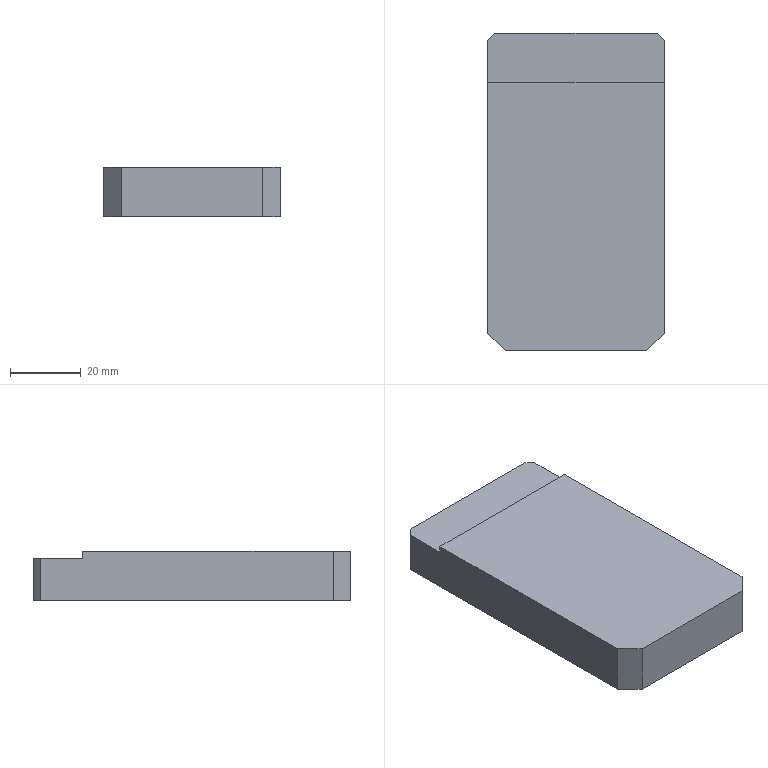Part | STEP file | Backup 2012-3-22-014 | 1 solid | 12 faces | box 50 x 90 x 14 mm | volume 61202 mm3 | plane 12
STEP:
#1=CARTESIAN_POINT('',(0.,0.,0.));
#2=DIRECTION('',(0.,0.,1.));
#3=DIRECTION('',(1.,0.,0.));
#4=AXIS2_PLACEMENT_3D('',#1,#2,#3);
#5=CARTESIAN_POINT('',(23.,45.,12.));
#6=VERTEX_POINT('',#5);
#7=CARTESIAN_POINT('',(-23.,45.,12.));
#8=VERTEX_POINT('',#7);
#9=CARTESIAN_POINT('',(-25.,45.,12.));
#10=DIRECTION('',(-1.,0.,0.));
#11=VECTOR('',#10,1.);
#12=LINE('',#9,#11);
#13=CARTESIAN_POINT('',(-25.,45.,14.));
#14=DIRECTION('',(0.,-1.,0.));
#15=DIRECTION('',(0.,0.,-1.));
#16=AXIS2_PLACEMENT_3D('',#13,#14,#15);
#17=PLANE('',#16);
#18=CARTESIAN_POINT('',(2.,0.));
#19=DIRECTION('',(0.,-1.));
#20=VECTOR('',#19,1.);
#21=LINE('',#18,#20);
#22=(GEOMETRIC_REPRESENTATION_CONTEXT(2)PARAMETRIC_REPRESENTATION_CONTEXT()REPRESENTATION_CONTEXT('',''));
#23=DEFINITIONAL_REPRESENTATION('',(#21),#22);
#24=PCURVE('',#17,#23);
#25=CARTESIAN_POINT('',(-25.,31.,12.));
#26=DIRECTION('',(0.,0.,1.));
#27=DIRECTION('',(1.,0.,0.));
#28=AXIS2_PLACEMENT_3D('',#25,#26,#27);
#29=PLANE('',#28);
#30=CARTESIAN_POINT('',(0.,14.));
#31=DIRECTION('',(-1.,0.));
#32=VECTOR('',#31,1.);
#33=LINE('',#30,#32);
#34=(GEOMETRIC_REPRESENTATION_CONTEXT(2)PARAMETRIC_REPRESENTATION_CONTEXT()REPRESENTATION_CONTEXT('',''));
#35=DEFINITIONAL_REPRESENTATION('',(#33),#34);
#36=PCURVE('',#29,#35);
#37=SURFACE_CURVE('',#12,(#24,#36),.PCURVE_S1.);
#38=EDGE_CURVE('',#6,#8,#37,.T.);
#39=ORIENTED_EDGE('',*,*,#38,.F.);
#40=CARTESIAN_POINT('',(23.,45.,0.));
#41=VERTEX_POINT('',#40);
#42=CARTESIAN_POINT('',(23.,45.,14.));
#43=DIRECTION('',(0.,0.,-1.));
#44=VECTOR('',#43,1.);
#45=LINE('',#42,#44);
#46=CARTESIAN_POINT('',(0.,48.));
#47=DIRECTION('',(1.,0.));
#48=VECTOR('',#47,1.);
#49=LINE('',#46,#48);
#50=(GEOMETRIC_REPRESENTATION_CONTEXT(2)PARAMETRIC_REPRESENTATION_CONTEXT()REPRESENTATION_CONTEXT('',''));
#51=DEFINITIONAL_REPRESENTATION('',(#49),#50);
#52=PCURVE('',#17,#51);
#53=CARTESIAN_POINT('',(23.,45.,14.));
#54=DIRECTION('',(-0.7071,-0.7071,0.));
#55=DIRECTION('',(0.7071,-0.7071,0.));
#56=AXIS2_PLACEMENT_3D('',#53,#54,#55);
#57=PLANE('',#56);
#58=CARTESIAN_POINT('',(0.,0.));
#59=DIRECTION('',(0.,-1.));
#60=VECTOR('',#59,1.);
#61=LINE('',#58,#60);
#62=(GEOMETRIC_REPRESENTATION_CONTEXT(2)PARAMETRIC_REPRESENTATION_CONTEXT()REPRESENTATION_CONTEXT('',''));
#63=DEFINITIONAL_REPRESENTATION('',(#61),#62);
#64=PCURVE('',#57,#63);
#65=SURFACE_CURVE('',#45,(#52,#64),.PCURVE_S1.);
#66=EDGE_CURVE('',#6,#41,#65,.T.);
#67=ORIENTED_EDGE('',*,*,#66,.T.);
#68=CARTESIAN_POINT('',(-23.,45.,0.));
#69=VERTEX_POINT('',#68);
#70=CARTESIAN_POINT('',(-25.,45.,0.));
#71=DIRECTION('',(-1.,0.,0.));
#72=VECTOR('',#71,1.);
#73=LINE('',#70,#72);
#74=CARTESIAN_POINT('',(14.,0.));
#75=DIRECTION('',(0.,-1.));
#76=VECTOR('',#75,1.);
#77=LINE('',#74,#76);
#78=(GEOMETRIC_REPRESENTATION_CONTEXT(2)PARAMETRIC_REPRESENTATION_CONTEXT()REPRESENTATION_CONTEXT('',''));
#79=DEFINITIONAL_REPRESENTATION('',(#77),#78);
#80=PCURVE('',#17,#79);
#81=CARTESIAN_POINT('',(25.,-45.,0.));
#82=DIRECTION('',(0.,0.,1.));
#83=DIRECTION('',(1.,0.,0.));
#84=AXIS2_PLACEMENT_3D('',#81,#82,#83);
#85=PLANE('',#84);
#86=CARTESIAN_POINT('',(-50.,90.));
#87=DIRECTION('',(-1.,0.));
#88=VECTOR('',#87,1.);
#89=LINE('',#86,#88);
#90=(GEOMETRIC_REPRESENTATION_CONTEXT(2)PARAMETRIC_REPRESENTATION_CONTEXT()REPRESENTATION_CONTEXT('',''));
#91=DEFINITIONAL_REPRESENTATION('',(#89),#90);
#92=PCURVE('',#85,#91);
#93=SURFACE_CURVE('',#73,(#80,#92),.PCURVE_S1.);
#94=EDGE_CURVE('',#41,#69,#93,.T.);
#95=ORIENTED_EDGE('',*,*,#94,.T.);
#96=CARTESIAN_POINT('',(-23.,45.,14.));
#97=DIRECTION('',(0.,0.,1.));
#98=VECTOR('',#97,1.);
#99=LINE('',#96,#98);
#100=CARTESIAN_POINT('',(0.,2.));
#101=DIRECTION('',(-1.,0.));
#102=VECTOR('',#101,1.);
#103=LINE('',#100,#102);
#104=(GEOMETRIC_REPRESENTATION_CONTEXT(2)PARAMETRIC_REPRESENTATION_CONTEXT()REPRESENTATION_CONTEXT('',''));
#105=DEFINITIONAL_REPRESENTATION('',(#103),#104);
#106=PCURVE('',#17,#105);
#107=CARTESIAN_POINT('',(-25.,43.,14.));
#108=DIRECTION('',(0.7071,-0.7071,0.));
#109=DIRECTION('',(0.7071,0.7071,0.));
#110=AXIS2_PLACEMENT_3D('',#107,#108,#109);
#111=PLANE('',#110);
#112=CARTESIAN_POINT('',(2.828,0.));
#113=DIRECTION('',(0.,1.));
#114=VECTOR('',#113,1.);
#115=LINE('',#112,#114);
#116=(GEOMETRIC_REPRESENTATION_CONTEXT(2)PARAMETRIC_REPRESENTATION_CONTEXT()REPRESENTATION_CONTEXT('',''));
#117=DEFINITIONAL_REPRESENTATION('',(#115),#116);
#118=PCURVE('',#111,#117);
#119=SURFACE_CURVE('',#99,(#106,#118),.PCURVE_S1.);
#120=EDGE_CURVE('',#69,#8,#119,.T.);
#121=ORIENTED_EDGE('',*,*,#120,.T.);
#122=EDGE_LOOP('',(#39,#67,#95,#121));
#123=FACE_BOUND('',#122,.T.);
#124=ADVANCED_FACE('',(#123),#17,.F.);
#125=CARTESIAN_POINT('',(25.,-40.,0.));
#126=VERTEX_POINT('',#125);
#127=CARTESIAN_POINT('',(25.,43.,0.));
#128=VERTEX_POINT('',#127);
#129=CARTESIAN_POINT('',(25.,45.,0.));
#130=DIRECTION('',(0.,1.,0.));
#131=VECTOR('',#130,1.);
#132=LINE('',#129,#131);
#133=CARTESIAN_POINT('',(25.,45.,14.));
#134=DIRECTION('',(-1.,0.,0.));
#135=DIRECTION('',(0.,-1.,0.));
#136=AXIS2_PLACEMENT_3D('',#133,#134,#135);
#137=PLANE('',#136);
#138=CARTESIAN_POINT('',(0.,-14.));
#139=DIRECTION('',(-1.,0.));
#140=VECTOR('',#139,1.);
#141=LINE('',#138,#140);
#142=(GEOMETRIC_REPRESENTATION_CONTEXT(2)PARAMETRIC_REPRESENTATION_CONTEXT()REPRESENTATION_CONTEXT('',''));
#143=DEFINITIONAL_REPRESENTATION('',(#141),#142);
#144=PCURVE('',#137,#143);
#145=CARTESIAN_POINT('',(0.,90.));
#146=DIRECTION('',(0.,1.));
#147=VECTOR('',#146,1.);
#148=LINE('',#145,#147);
#149=(GEOMETRIC_REPRESENTATION_CONTEXT(2)PARAMETRIC_REPRESENTATION_CONTEXT()REPRESENTATION_CONTEXT('',''));
#150=DEFINITIONAL_REPRESENTATION('',(#148),#149);
#151=PCURVE('',#85,#150);
#152=SURFACE_CURVE('',#132,(#144,#151),.PCURVE_S1.);
#153=EDGE_CURVE('',#126,#128,#152,.T.);
#154=ORIENTED_EDGE('',*,*,#153,.T.);
#155=CARTESIAN_POINT('',(25.,43.,12.));
#156=VERTEX_POINT('',#155);
#157=CARTESIAN_POINT('',(25.,43.,14.));
#158=DIRECTION('',(0.,0.,1.));
#159=VECTOR('',#158,1.);
#160=LINE('',#157,#159);
#161=CARTESIAN_POINT('',(2.,0.));
#162=DIRECTION('',(0.,1.));
#163=VECTOR('',#162,1.);
#164=LINE('',#161,#163);
#165=(GEOMETRIC_REPRESENTATION_CONTEXT(2)PARAMETRIC_REPRESENTATION_CONTEXT()REPRESENTATION_CONTEXT('',''));
#166=DEFINITIONAL_REPRESENTATION('',(#164),#165);
#167=PCURVE('',#137,#166);
#168=CARTESIAN_POINT('',(2.828,0.));
#169=DIRECTION('',(0.,1.));
#170=VECTOR('',#169,1.);
#171=LINE('',#168,#170);
#172=(GEOMETRIC_REPRESENTATION_CONTEXT(2)PARAMETRIC_REPRESENTATION_CONTEXT()REPRESENTATION_CONTEXT('',''));
#173=DEFINITIONAL_REPRESENTATION('',(#171),#172);
#174=PCURVE('',#57,#173);
#175=SURFACE_CURVE('',#160,(#167,#174),.PCURVE_S1.);
#176=EDGE_CURVE('',#128,#156,#175,.T.);
#177=ORIENTED_EDGE('',*,*,#176,.T.);
#178=CARTESIAN_POINT('',(25.,31.,12.));
#179=VERTEX_POINT('',#178);
#180=CARTESIAN_POINT('',(25.,45.,12.));
#181=DIRECTION('',(0.,1.,0.));
#182=VECTOR('',#181,1.);
#183=LINE('',#180,#182);
#184=CARTESIAN_POINT('',(0.,-2.));
#185=DIRECTION('',(-1.,0.));
#186=VECTOR('',#185,1.);
#187=LINE('',#184,#186);
#188=(GEOMETRIC_REPRESENTATION_CONTEXT(2)PARAMETRIC_REPRESENTATION_CONTEXT()REPRESENTATION_CONTEXT('',''));
#189=DEFINITIONAL_REPRESENTATION('',(#187),#188);
#190=PCURVE('',#137,#189);
#191=CARTESIAN_POINT('',(50.,14.));
#192=DIRECTION('',(0.,1.));
#193=VECTOR('',#192,1.);
#194=LINE('',#191,#193);
#195=(GEOMETRIC_REPRESENTATION_CONTEXT(2)PARAMETRIC_REPRESENTATION_CONTEXT()REPRESENTATION_CONTEXT('',''));
#196=DEFINITIONAL_REPRESENTATION('',(#194),#195);
#197=PCURVE('',#29,#196);
#198=SURFACE_CURVE('',#183,(#190,#197),.PCURVE_S1.);
#199=EDGE_CURVE('',#179,#156,#198,.T.);
#200=ORIENTED_EDGE('',*,*,#199,.F.);
#201=CARTESIAN_POINT('',(25.,31.,14.));
#202=VERTEX_POINT('',#201);
#203=CARTESIAN_POINT('',(25.,31.,12.));
#204=DIRECTION('',(0.,0.,1.));
#205=VECTOR('',#204,1.);
#206=LINE('',#203,#205);
#207=CARTESIAN_POINT('',(14.,-2.));
#208=DIRECTION('',(0.,1.));
#209=VECTOR('',#208,1.);
#210=LINE('',#207,#209);
#211=(GEOMETRIC_REPRESENTATION_CONTEXT(2)PARAMETRIC_REPRESENTATION_CONTEXT()REPRESENTATION_CONTEXT('',''));
#212=DEFINITIONAL_REPRESENTATION('',(#210),#211);
#213=PCURVE('',#137,#212);
#214=CARTESIAN_POINT('',(-25.,31.,12.));
#215=DIRECTION('',(0.,-1.,0.));
#216=DIRECTION('',(0.,0.,-1.));
#217=AXIS2_PLACEMENT_3D('',#214,#215,#216);
#218=PLANE('',#217);
#219=CARTESIAN_POINT('',(0.,50.));
#220=DIRECTION('',(-1.,0.));
#221=VECTOR('',#220,1.);
#222=LINE('',#219,#221);
#223=(GEOMETRIC_REPRESENTATION_CONTEXT(2)PARAMETRIC_REPRESENTATION_CONTEXT()REPRESENTATION_CONTEXT('',''));
#224=DEFINITIONAL_REPRESENTATION('',(#222),#223);
#225=PCURVE('',#218,#224);
#226=SURFACE_CURVE('',#206,(#213,#225),.PCURVE_S1.);
#227=EDGE_CURVE('',#179,#202,#226,.T.);
#228=ORIENTED_EDGE('',*,*,#227,.T.);
#229=CARTESIAN_POINT('',(25.,-40.,14.));
#230=VERTEX_POINT('',#229);
#231=CARTESIAN_POINT('',(25.,45.,14.));
#232=DIRECTION('',(0.,1.,0.));
#233=VECTOR('',#232,1.);
#234=LINE('',#231,#233);
#235=CARTESIAN_POINT('',(0.,0.));
#236=DIRECTION('',(-1.,0.));
#237=VECTOR('',#236,1.);
#238=LINE('',#235,#237);
#239=(GEOMETRIC_REPRESENTATION_CONTEXT(2)PARAMETRIC_REPRESENTATION_CONTEXT()REPRESENTATION_CONTEXT('',''));
#240=DEFINITIONAL_REPRESENTATION('',(#238),#239);
#241=PCURVE('',#137,#240);
#242=CARTESIAN_POINT('',(25.,-45.,14.));
#243=DIRECTION('',(0.,0.,1.));
#244=DIRECTION('',(1.,0.,0.));
#245=AXIS2_PLACEMENT_3D('',#242,#243,#244);
#246=PLANE('',#245);
#247=CARTESIAN_POINT('',(0.,90.));
#248=DIRECTION('',(0.,1.));
#249=VECTOR('',#248,1.);
#250=LINE('',#247,#249);
#251=(GEOMETRIC_REPRESENTATION_CONTEXT(2)PARAMETRIC_REPRESENTATION_CONTEXT()REPRESENTATION_CONTEXT('',''));
#252=DEFINITIONAL_REPRESENTATION('',(#250),#251);
#253=PCURVE('',#246,#252);
#254=SURFACE_CURVE('',#234,(#241,#253),.PCURVE_S1.);
#255=EDGE_CURVE('',#230,#202,#254,.T.);
#256=ORIENTED_EDGE('',*,*,#255,.F.);
#257=CARTESIAN_POINT('',(25.,-40.,14.));
#258=DIRECTION('',(0.,0.,-1.));
#259=VECTOR('',#258,1.);
#260=LINE('',#257,#259);
#261=CARTESIAN_POINT('',(85.,0.));
#262=DIRECTION('',(0.,-1.));
#263=VECTOR('',#262,1.);
#264=LINE('',#261,#263);
#265=(GEOMETRIC_REPRESENTATION_CONTEXT(2)PARAMETRIC_REPRESENTATION_CONTEXT()REPRESENTATION_CONTEXT('',''));
#266=DEFINITIONAL_REPRESENTATION('',(#264),#265);
#267=PCURVE('',#137,#266);
#268=CARTESIAN_POINT('',(25.,-40.,14.));
#269=DIRECTION('',(-0.7071,0.7071,0.));
#270=DIRECTION('',(-0.7071,-0.7071,0.));
#271=AXIS2_PLACEMENT_3D('',#268,#269,#270);
#272=PLANE('',#271);
#273=CARTESIAN_POINT('',(0.,0.));
#274=DIRECTION('',(0.,-1.));
#275=VECTOR('',#274,1.);
#276=LINE('',#273,#275);
#277=(GEOMETRIC_REPRESENTATION_CONTEXT(2)PARAMETRIC_REPRESENTATION_CONTEXT()REPRESENTATION_CONTEXT('',''));
#278=DEFINITIONAL_REPRESENTATION('',(#276),#277);
#279=PCURVE('',#272,#278);
#280=SURFACE_CURVE('',#260,(#267,#279),.PCURVE_S1.);
#281=EDGE_CURVE('',#230,#126,#280,.T.);
#282=ORIENTED_EDGE('',*,*,#281,.T.);
#283=EDGE_LOOP('',(#154,#177,#200,#228,#256,#282));
#284=FACE_BOUND('',#283,.T.);
#285=ADVANCED_FACE('',(#284),#137,.F.);
#286=CARTESIAN_POINT('',(-25.,43.,12.));
#287=VERTEX_POINT('',#286);
#288=CARTESIAN_POINT('',(-25.,31.,12.));
#289=VERTEX_POINT('',#288);
#290=CARTESIAN_POINT('',(-25.,45.,12.));
#291=DIRECTION('',(0.,-1.,0.));
#292=VECTOR('',#291,1.);
#293=LINE('',#290,#292);
#294=CARTESIAN_POINT('',(-25.,45.,14.));
#295=DIRECTION('',(1.,0.,0.));
#296=DIRECTION('',(0.,1.,0.));
#297=AXIS2_PLACEMENT_3D('',#294,#295,#296);
#298=PLANE('',#297);
#299=CARTESIAN_POINT('',(0.,-2.));
#300=DIRECTION('',(-1.,0.));
#301=VECTOR('',#300,1.);
#302=LINE('',#299,#301);
#303=(GEOMETRIC_REPRESENTATION_CONTEXT(2)PARAMETRIC_REPRESENTATION_CONTEXT()REPRESENTATION_CONTEXT('',''));
#304=DEFINITIONAL_REPRESENTATION('',(#302),#303);
#305=PCURVE('',#298,#304);
#306=CARTESIAN_POINT('',(0.,14.));
#307=DIRECTION('',(0.,-1.));
#308=VECTOR('',#307,1.);
#309=LINE('',#306,#308);
#310=(GEOMETRIC_REPRESENTATION_CONTEXT(2)PARAMETRIC_REPRESENTATION_CONTEXT()REPRESENTATION_CONTEXT('',''));
#311=DEFINITIONAL_REPRESENTATION('',(#309),#310);
#312=PCURVE('',#29,#311);
#313=SURFACE_CURVE('',#293,(#305,#312),.PCURVE_S1.);
#314=EDGE_CURVE('',#287,#289,#313,.T.);
#315=ORIENTED_EDGE('',*,*,#314,.F.);
#316=CARTESIAN_POINT('',(-25.,43.,0.));
#317=VERTEX_POINT('',#316);
#318=CARTESIAN_POINT('',(-25.,43.,14.));
#319=DIRECTION('',(0.,0.,-1.));
#320=VECTOR('',#319,1.);
#321=LINE('',#318,#320);
#322=CARTESIAN_POINT('',(-2.,0.));
#323=DIRECTION('',(0.,-1.));
#324=VECTOR('',#323,1.);
#325=LINE('',#322,#324);
#326=(GEOMETRIC_REPRESENTATION_CONTEXT(2)PARAMETRIC_REPRESENTATION_CONTEXT()REPRESENTATION_CONTEXT('',''));
#327=DEFINITIONAL_REPRESENTATION('',(#325),#326);
#328=PCURVE('',#298,#327);
#329=CARTESIAN_POINT('',(0.,0.));
#330=DIRECTION('',(0.,-1.));
#331=VECTOR('',#330,1.);
#332=LINE('',#329,#331);
#333=(GEOMETRIC_REPRESENTATION_CONTEXT(2)PARAMETRIC_REPRESENTATION_CONTEXT()REPRESENTATION_CONTEXT('',''));
#334=DEFINITIONAL_REPRESENTATION('',(#332),#333);
#335=PCURVE('',#111,#334);
#336=SURFACE_CURVE('',#321,(#328,#335),.PCURVE_S1.);
#337=EDGE_CURVE('',#287,#317,#336,.T.);
#338=ORIENTED_EDGE('',*,*,#337,.T.);
#339=CARTESIAN_POINT('',(-25.,-40.,0.));
#340=VERTEX_POINT('',#339);
#341=CARTESIAN_POINT('',(-25.,45.,0.));
#342=DIRECTION('',(0.,-1.,0.));
#343=VECTOR('',#342,1.);
#344=LINE('',#341,#343);
#345=CARTESIAN_POINT('',(0.,-14.));
#346=DIRECTION('',(-1.,0.));
#347=VECTOR('',#346,1.);
#348=LINE('',#345,#347);
#349=(GEOMETRIC_REPRESENTATION_CONTEXT(2)PARAMETRIC_REPRESENTATION_CONTEXT()REPRESENTATION_CONTEXT('',''));
#350=DEFINITIONAL_REPRESENTATION('',(#348),#349);
#351=PCURVE('',#298,#350);
#352=CARTESIAN_POINT('',(-50.,90.));
#353=DIRECTION('',(0.,-1.));
#354=VECTOR('',#353,1.);
#355=LINE('',#352,#354);
#356=(GEOMETRIC_REPRESENTATION_CONTEXT(2)PARAMETRIC_REPRESENTATION_CONTEXT()REPRESENTATION_CONTEXT('',''));
#357=DEFINITIONAL_REPRESENTATION('',(#355),#356);
#358=PCURVE('',#85,#357);
#359=SURFACE_CURVE('',#344,(#351,#358),.PCURVE_S1.);
#360=EDGE_CURVE('',#317,#340,#359,.T.);
#361=ORIENTED_EDGE('',*,*,#360,.T.);
#362=CARTESIAN_POINT('',(-25.,-40.,14.));
#363=VERTEX_POINT('',#362);
#364=CARTESIAN_POINT('',(-25.,-40.,14.));
#365=DIRECTION('',(0.,0.,1.));
#366=VECTOR('',#365,1.);
#367=LINE('',#364,#366);
#368=CARTESIAN_POINT('',(-85.,0.));
#369=DIRECTION('',(0.,1.));
#370=VECTOR('',#369,1.);
#371=LINE('',#368,#370);
#372=(GEOMETRIC_REPRESENTATION_CONTEXT(2)PARAMETRIC_REPRESENTATION_CONTEXT()REPRESENTATION_CONTEXT('',''));
#373=DEFINITIONAL_REPRESENTATION('',(#371),#372);
#374=PCURVE('',#298,#373);
#375=CARTESIAN_POINT('',(-20.,-45.,14.));
#376=DIRECTION('',(0.7071,0.7071,0.));
#377=DIRECTION('',(-0.7071,0.7071,0.));
#378=AXIS2_PLACEMENT_3D('',#375,#376,#377);
#379=PLANE('',#378);
#380=CARTESIAN_POINT('',(7.071,0.));
#381=DIRECTION('',(0.,1.));
#382=VECTOR('',#381,1.);
#383=LINE('',#380,#382);
#384=(GEOMETRIC_REPRESENTATION_CONTEXT(2)PARAMETRIC_REPRESENTATION_CONTEXT()REPRESENTATION_CONTEXT('',''));
#385=DEFINITIONAL_REPRESENTATION('',(#383),#384);
#386=PCURVE('',#379,#385);
#387=SURFACE_CURVE('',#367,(#374,#386),.PCURVE_S1.);
#388=EDGE_CURVE('',#340,#363,#387,.T.);
#389=ORIENTED_EDGE('',*,*,#388,.T.);
#390=CARTESIAN_POINT('',(-25.,31.,14.));
#391=VERTEX_POINT('',#390);
#392=CARTESIAN_POINT('',(-25.,45.,14.));
#393=DIRECTION('',(0.,-1.,0.));
#394=VECTOR('',#393,1.);
#395=LINE('',#392,#394);
#396=CARTESIAN_POINT('',(0.,0.));
#397=DIRECTION('',(-1.,0.));
#398=VECTOR('',#397,1.);
#399=LINE('',#396,#398);
#400=(GEOMETRIC_REPRESENTATION_CONTEXT(2)PARAMETRIC_REPRESENTATION_CONTEXT()REPRESENTATION_CONTEXT('',''));
#401=DEFINITIONAL_REPRESENTATION('',(#399),#400);
#402=PCURVE('',#298,#401);
#403=CARTESIAN_POINT('',(-50.,90.));
#404=DIRECTION('',(0.,-1.));
#405=VECTOR('',#404,1.);
#406=LINE('',#403,#405);
#407=(GEOMETRIC_REPRESENTATION_CONTEXT(2)PARAMETRIC_REPRESENTATION_CONTEXT()REPRESENTATION_CONTEXT('',''));
#408=DEFINITIONAL_REPRESENTATION('',(#406),#407);
#409=PCURVE('',#246,#408);
#410=SURFACE_CURVE('',#395,(#402,#409),.PCURVE_S1.);
#411=EDGE_CURVE('',#391,#363,#410,.T.);
#412=ORIENTED_EDGE('',*,*,#411,.F.);
#413=CARTESIAN_POINT('',(-25.,31.,12.));
#414=DIRECTION('',(0.,0.,1.));
#415=VECTOR('',#414,1.);
#416=LINE('',#413,#415);
#417=CARTESIAN_POINT('',(-14.,-2.));
#418=DIRECTION('',(0.,1.));
#419=VECTOR('',#418,1.);
#420=LINE('',#417,#419);
#421=(GEOMETRIC_REPRESENTATION_CONTEXT(2)PARAMETRIC_REPRESENTATION_CONTEXT()REPRESENTATION_CONTEXT('',''));
#422=DEFINITIONAL_REPRESENTATION('',(#420),#421);
#423=PCURVE('',#298,#422);
#424=CARTESIAN_POINT('',(0.,0.));
#425=DIRECTION('',(-1.,0.));
#426=VECTOR('',#425,1.);
#427=LINE('',#424,#426);
#428=(GEOMETRIC_REPRESENTATION_CONTEXT(2)PARAMETRIC_REPRESENTATION_CONTEXT()REPRESENTATION_CONTEXT('',''));
#429=DEFINITIONAL_REPRESENTATION('',(#427),#428);
#430=PCURVE('',#218,#429);
#431=SURFACE_CURVE('',#416,(#423,#430),.PCURVE_S1.);
#432=EDGE_CURVE('',#289,#391,#431,.T.);
#433=ORIENTED_EDGE('',*,*,#432,.F.);
#434=EDGE_LOOP('',(#315,#338,#361,#389,#412,#433));
#435=FACE_BOUND('',#434,.T.);
#436=ADVANCED_FACE('',(#435),#298,.F.);
#437=CARTESIAN_POINT('',(-20.,-45.,0.));
#438=VERTEX_POINT('',#437);
#439=CARTESIAN_POINT('',(20.,-45.,0.));
#440=VERTEX_POINT('',#439);
#441=CARTESIAN_POINT('',(-25.,-45.,0.));
#442=DIRECTION('',(1.,0.,0.));
#443=VECTOR('',#442,1.);
#444=LINE('',#441,#443);
#445=CARTESIAN_POINT('',(-25.,-45.,14.));
#446=DIRECTION('',(0.,1.,0.));
#447=DIRECTION('',(0.,0.,1.));
#448=AXIS2_PLACEMENT_3D('',#445,#446,#447);
#449=PLANE('',#448);
#450=CARTESIAN_POINT('',(-14.,0.));
#451=DIRECTION('',(0.,1.));
#452=VECTOR('',#451,1.);
#453=LINE('',#450,#452);
#454=(GEOMETRIC_REPRESENTATION_CONTEXT(2)PARAMETRIC_REPRESENTATION_CONTEXT()REPRESENTATION_CONTEXT('',''));
#455=DEFINITIONAL_REPRESENTATION('',(#453),#454);
#456=PCURVE('',#449,#455);
#457=CARTESIAN_POINT('',(-50.,0.));
#458=DIRECTION('',(1.,0.));
#459=VECTOR('',#458,1.);
#460=LINE('',#457,#459);
#461=(GEOMETRIC_REPRESENTATION_CONTEXT(2)PARAMETRIC_REPRESENTATION_CONTEXT()REPRESENTATION_CONTEXT('',''));
#462=DEFINITIONAL_REPRESENTATION('',(#460),#461);
#463=PCURVE('',#85,#462);
#464=SURFACE_CURVE('',#444,(#456,#463),.PCURVE_S1.);
#465=EDGE_CURVE('',#438,#440,#464,.T.);
#466=ORIENTED_EDGE('',*,*,#465,.T.);
#467=CARTESIAN_POINT('',(20.,-45.,14.));
#468=VERTEX_POINT('',#467);
#469=CARTESIAN_POINT('',(20.,-45.,14.));
#470=DIRECTION('',(0.,0.,1.));
#471=VECTOR('',#470,1.);
#472=LINE('',#469,#471);
#473=CARTESIAN_POINT('',(0.,45.));
#474=DIRECTION('',(1.,0.));
#475=VECTOR('',#474,1.);
#476=LINE('',#473,#475);
#477=(GEOMETRIC_REPRESENTATION_CONTEXT(2)PARAMETRIC_REPRESENTATION_CONTEXT()REPRESENTATION_CONTEXT('',''));
#478=DEFINITIONAL_REPRESENTATION('',(#476),#477);
#479=PCURVE('',#449,#478);
#480=CARTESIAN_POINT('',(7.071,0.));
#481=DIRECTION('',(0.,1.));
#482=VECTOR('',#481,1.);
#483=LINE('',#480,#482);
#484=(GEOMETRIC_REPRESENTATION_CONTEXT(2)PARAMETRIC_REPRESENTATION_CONTEXT()REPRESENTATION_CONTEXT('',''));
#485=DEFINITIONAL_REPRESENTATION('',(#483),#484);
#486=PCURVE('',#272,#485);
#487=SURFACE_CURVE('',#472,(#479,#486),.PCURVE_S1.);
#488=EDGE_CURVE('',#440,#468,#487,.T.);
#489=ORIENTED_EDGE('',*,*,#488,.T.);
#490=CARTESIAN_POINT('',(-20.,-45.,14.));
#491=VERTEX_POINT('',#490);
#492=CARTESIAN_POINT('',(-25.,-45.,14.));
#493=DIRECTION('',(1.,0.,0.));
#494=VECTOR('',#493,1.);
#495=LINE('',#492,#494);
#496=CARTESIAN_POINT('',(0.,0.));
#497=DIRECTION('',(0.,1.));
#498=VECTOR('',#497,1.);
#499=LINE('',#496,#498);
#500=(GEOMETRIC_REPRESENTATION_CONTEXT(2)PARAMETRIC_REPRESENTATION_CONTEXT()REPRESENTATION_CONTEXT('',''));
#501=DEFINITIONAL_REPRESENTATION('',(#499),#500);
#502=PCURVE('',#449,#501);
#503=CARTESIAN_POINT('',(-50.,0.));
#504=DIRECTION('',(1.,0.));
#505=VECTOR('',#504,1.);
#506=LINE('',#503,#505);
#507=(GEOMETRIC_REPRESENTATION_CONTEXT(2)PARAMETRIC_REPRESENTATION_CONTEXT()REPRESENTATION_CONTEXT('',''));
#508=DEFINITIONAL_REPRESENTATION('',(#506),#507);
#509=PCURVE('',#246,#508);
#510=SURFACE_CURVE('',#495,(#502,#509),.PCURVE_S1.);
#511=EDGE_CURVE('',#491,#468,#510,.T.);
#512=ORIENTED_EDGE('',*,*,#511,.F.);
#513=CARTESIAN_POINT('',(-20.,-45.,14.));
#514=DIRECTION('',(0.,0.,-1.));
#515=VECTOR('',#514,1.);
#516=LINE('',#513,#515);
#517=CARTESIAN_POINT('',(0.,5.));
#518=DIRECTION('',(-1.,0.));
#519=VECTOR('',#518,1.);
#520=LINE('',#517,#519);
#521=(GEOMETRIC_REPRESENTATION_CONTEXT(2)PARAMETRIC_REPRESENTATION_CONTEXT()REPRESENTATION_CONTEXT('',''));
#522=DEFINITIONAL_REPRESENTATION('',(#520),#521);
#523=PCURVE('',#449,#522);
#524=CARTESIAN_POINT('',(0.,0.));
#525=DIRECTION('',(0.,-1.));
#526=VECTOR('',#525,1.);
#527=LINE('',#524,#526);
#528=(GEOMETRIC_REPRESENTATION_CONTEXT(2)PARAMETRIC_REPRESENTATION_CONTEXT()REPRESENTATION_CONTEXT('',''));
#529=DEFINITIONAL_REPRESENTATION('',(#527),#528);
#530=PCURVE('',#379,#529);
#531=SURFACE_CURVE('',#516,(#523,#530),.PCURVE_S1.);
#532=EDGE_CURVE('',#491,#438,#531,.T.);
#533=ORIENTED_EDGE('',*,*,#532,.T.);
#534=EDGE_LOOP('',(#466,#489,#512,#533));
#535=FACE_BOUND('',#534,.T.);
#536=ADVANCED_FACE('',(#535),#449,.F.);
#537=ORIENTED_EDGE('',*,*,#511,.T.);
#538=CARTESIAN_POINT('',(22.5,-42.5,14.));
#539=DIRECTION('',(0.7071,0.7071,0.));
#540=VECTOR('',#539,1.);
#541=LINE('',#538,#540);
#542=CARTESIAN_POINT('',(-2.5,2.5));
#543=DIRECTION('',(0.7071,0.7071));
#544=VECTOR('',#543,1.);
#545=LINE('',#542,#544);
#546=(GEOMETRIC_REPRESENTATION_CONTEXT(2)PARAMETRIC_REPRESENTATION_CONTEXT()REPRESENTATION_CONTEXT('',''));
#547=DEFINITIONAL_REPRESENTATION('',(#545),#546);
#548=PCURVE('',#246,#547);
#549=CARTESIAN_POINT('',(3.536,0.));
#550=DIRECTION('',(-1.,0.));
#551=VECTOR('',#550,1.);
#552=LINE('',#549,#551);
#553=(GEOMETRIC_REPRESENTATION_CONTEXT(2)PARAMETRIC_REPRESENTATION_CONTEXT()REPRESENTATION_CONTEXT('',''));
#554=DEFINITIONAL_REPRESENTATION('',(#552),#553);
#555=PCURVE('',#272,#554);
#556=SURFACE_CURVE('',#541,(#548,#555),.PCURVE_S1.);
#557=EDGE_CURVE('',#468,#230,#556,.T.);
#558=ORIENTED_EDGE('',*,*,#557,.T.);
#559=ORIENTED_EDGE('',*,*,#255,.T.);
#560=CARTESIAN_POINT('',(-25.,31.,14.));
#561=DIRECTION('',(1.,0.,0.));
#562=VECTOR('',#561,1.);
#563=LINE('',#560,#562);
#564=CARTESIAN_POINT('',(-50.,76.));
#565=DIRECTION('',(1.,0.));
#566=VECTOR('',#565,1.);
#567=LINE('',#564,#566);
#568=(GEOMETRIC_REPRESENTATION_CONTEXT(2)PARAMETRIC_REPRESENTATION_CONTEXT()REPRESENTATION_CONTEXT('',''));
#569=DEFINITIONAL_REPRESENTATION('',(#567),#568);
#570=PCURVE('',#246,#569);
#571=CARTESIAN_POINT('',(-2.,0.));
#572=DIRECTION('',(0.,1.));
#573=VECTOR('',#572,1.);
#574=LINE('',#571,#573);
#575=(GEOMETRIC_REPRESENTATION_CONTEXT(2)PARAMETRIC_REPRESENTATION_CONTEXT()REPRESENTATION_CONTEXT('',''));
#576=DEFINITIONAL_REPRESENTATION('',(#574),#575);
#577=PCURVE('',#218,#576);
#578=SURFACE_CURVE('',#563,(#570,#577),.PCURVE_S1.);
#579=EDGE_CURVE('',#391,#202,#578,.T.);
#580=ORIENTED_EDGE('',*,*,#579,.F.);
#581=ORIENTED_EDGE('',*,*,#411,.T.);
#582=CARTESIAN_POINT('',(2.5,-67.5,14.));
#583=DIRECTION('',(0.7071,-0.7071,0.));
#584=VECTOR('',#583,1.);
#585=LINE('',#582,#584);
#586=CARTESIAN_POINT('',(-22.5,-22.5));
#587=DIRECTION('',(0.7071,-0.7071));
#588=VECTOR('',#587,1.);
#589=LINE('',#586,#588);
#590=(GEOMETRIC_REPRESENTATION_CONTEXT(2)PARAMETRIC_REPRESENTATION_CONTEXT()REPRESENTATION_CONTEXT('',''));
#591=DEFINITIONAL_REPRESENTATION('',(#589),#590);
#592=PCURVE('',#246,#591);
#593=CARTESIAN_POINT('',(-31.82,0.));
#594=DIRECTION('',(-1.,0.));
#595=VECTOR('',#594,1.);
#596=LINE('',#593,#595);
#597=(GEOMETRIC_REPRESENTATION_CONTEXT(2)PARAMETRIC_REPRESENTATION_CONTEXT()REPRESENTATION_CONTEXT('',''));
#598=DEFINITIONAL_REPRESENTATION('',(#596),#597);
#599=PCURVE('',#379,#598);
#600=SURFACE_CURVE('',#585,(#592,#599),.PCURVE_S1.);
#601=EDGE_CURVE('',#363,#491,#600,.T.);
#602=ORIENTED_EDGE('',*,*,#601,.T.);
#603=EDGE_LOOP('',(#537,#558,#559,#580,#581,#602));
#604=FACE_BOUND('',#603,.T.);
#605=ADVANCED_FACE('',(#604),#246,.T.);
#606=ORIENTED_EDGE('',*,*,#94,.F.);
#607=CARTESIAN_POINT('',(23.,45.,0.));
#608=DIRECTION('',(0.7071,-0.7071,0.));
#609=VECTOR('',#608,1.);
#610=LINE('',#607,#609);
#611=CARTESIAN_POINT('',(-2.,90.));
#612=DIRECTION('',(0.7071,-0.7071));
#613=VECTOR('',#612,1.);
#614=LINE('',#611,#613);
#615=(GEOMETRIC_REPRESENTATION_CONTEXT(2)PARAMETRIC_REPRESENTATION_CONTEXT()REPRESENTATION_CONTEXT('',''));
#616=DEFINITIONAL_REPRESENTATION('',(#614),#615);
#617=PCURVE('',#85,#616);
#618=CARTESIAN_POINT('',(0.,-14.));
#619=DIRECTION('',(1.,0.));
#620=VECTOR('',#619,1.);
#621=LINE('',#618,#620);
#622=(GEOMETRIC_REPRESENTATION_CONTEXT(2)PARAMETRIC_REPRESENTATION_CONTEXT()REPRESENTATION_CONTEXT('',''));
#623=DEFINITIONAL_REPRESENTATION('',(#621),#622);
#624=PCURVE('',#57,#623);
#625=SURFACE_CURVE('',#610,(#617,#624),.PCURVE_S1.);
#626=EDGE_CURVE('',#41,#128,#625,.T.);
#627=ORIENTED_EDGE('',*,*,#626,.T.);
#628=ORIENTED_EDGE('',*,*,#153,.F.);
#629=CARTESIAN_POINT('',(25.,-40.,0.));
#630=DIRECTION('',(-0.7071,-0.7071,0.));
#631=VECTOR('',#630,1.);
#632=LINE('',#629,#631);
#633=CARTESIAN_POINT('',(0.,5.));
#634=DIRECTION('',(-0.7071,-0.7071));
#635=VECTOR('',#634,1.);
#636=LINE('',#633,#635);
#637=(GEOMETRIC_REPRESENTATION_CONTEXT(2)PARAMETRIC_REPRESENTATION_CONTEXT()REPRESENTATION_CONTEXT('',''));
#638=DEFINITIONAL_REPRESENTATION('',(#636),#637);
#639=PCURVE('',#85,#638);
#640=CARTESIAN_POINT('',(0.,-14.));
#641=DIRECTION('',(1.,0.));
#642=VECTOR('',#641,1.);
#643=LINE('',#640,#642);
#644=(GEOMETRIC_REPRESENTATION_CONTEXT(2)PARAMETRIC_REPRESENTATION_CONTEXT()REPRESENTATION_CONTEXT('',''));
#645=DEFINITIONAL_REPRESENTATION('',(#643),#644);
#646=PCURVE('',#272,#645);
#647=SURFACE_CURVE('',#632,(#639,#646),.PCURVE_S1.);
#648=EDGE_CURVE('',#126,#440,#647,.T.);
#649=ORIENTED_EDGE('',*,*,#648,.T.);
#650=ORIENTED_EDGE('',*,*,#465,.F.);
#651=CARTESIAN_POINT('',(-20.,-45.,0.));
#652=DIRECTION('',(-0.7071,0.7071,0.));
#653=VECTOR('',#652,1.);
#654=LINE('',#651,#653);
#655=CARTESIAN_POINT('',(-45.,0.));
#656=DIRECTION('',(-0.7071,0.7071));
#657=VECTOR('',#656,1.);
#658=LINE('',#655,#657);
#659=(GEOMETRIC_REPRESENTATION_CONTEXT(2)PARAMETRIC_REPRESENTATION_CONTEXT()REPRESENTATION_CONTEXT('',''));
#660=DEFINITIONAL_REPRESENTATION('',(#658),#659);
#661=PCURVE('',#85,#660);
#662=CARTESIAN_POINT('',(0.,-14.));
#663=DIRECTION('',(1.,0.));
#664=VECTOR('',#663,1.);
#665=LINE('',#662,#664);
#666=(GEOMETRIC_REPRESENTATION_CONTEXT(2)PARAMETRIC_REPRESENTATION_CONTEXT()REPRESENTATION_CONTEXT('',''));
#667=DEFINITIONAL_REPRESENTATION('',(#665),#666);
#668=PCURVE('',#379,#667);
#669=SURFACE_CURVE('',#654,(#661,#668),.PCURVE_S1.);
#670=EDGE_CURVE('',#438,#340,#669,.T.);
#671=ORIENTED_EDGE('',*,*,#670,.T.);
#672=ORIENTED_EDGE('',*,*,#360,.F.);
#673=CARTESIAN_POINT('',(-25.,43.,0.));
#674=DIRECTION('',(0.7071,0.7071,0.));
#675=VECTOR('',#674,1.);
#676=LINE('',#673,#675);
#677=CARTESIAN_POINT('',(-50.,88.));
#678=DIRECTION('',(0.7071,0.7071));
#679=VECTOR('',#678,1.);
#680=LINE('',#677,#679);
#681=(GEOMETRIC_REPRESENTATION_CONTEXT(2)PARAMETRIC_REPRESENTATION_CONTEXT()REPRESENTATION_CONTEXT('',''));
#682=DEFINITIONAL_REPRESENTATION('',(#680),#681);
#683=PCURVE('',#85,#682);
#684=CARTESIAN_POINT('',(0.,-14.));
#685=DIRECTION('',(1.,0.));
#686=VECTOR('',#685,1.);
#687=LINE('',#684,#686);
#688=(GEOMETRIC_REPRESENTATION_CONTEXT(2)PARAMETRIC_REPRESENTATION_CONTEXT()REPRESENTATION_CONTEXT('',''));
#689=DEFINITIONAL_REPRESENTATION('',(#687),#688);
#690=PCURVE('',#111,#689);
#691=SURFACE_CURVE('',#676,(#683,#690),.PCURVE_S1.);
#692=EDGE_CURVE('',#317,#69,#691,.T.);
#693=ORIENTED_EDGE('',*,*,#692,.T.);
#694=EDGE_LOOP('',(#606,#627,#628,#649,#650,#671,#672,#693));
#695=FACE_BOUND('',#694,.T.);
#696=ADVANCED_FACE('',(#695),#85,.F.);
#697=ORIENTED_EDGE('',*,*,#579,.T.);
#698=ORIENTED_EDGE('',*,*,#227,.F.);
#699=CARTESIAN_POINT('',(-25.,31.,12.));
#700=DIRECTION('',(1.,0.,0.));
#701=VECTOR('',#700,1.);
#702=LINE('',#699,#701);
#703=CARTESIAN_POINT('',(0.,0.));
#704=DIRECTION('',(0.,1.));
#705=VECTOR('',#704,1.);
#706=LINE('',#703,#705);
#707=(GEOMETRIC_REPRESENTATION_CONTEXT(2)PARAMETRIC_REPRESENTATION_CONTEXT()REPRESENTATION_CONTEXT('',''));
#708=DEFINITIONAL_REPRESENTATION('',(#706),#707);
#709=PCURVE('',#218,#708);
#710=CARTESIAN_POINT('',(0.,0.));
#711=DIRECTION('',(1.,0.));
#712=VECTOR('',#711,1.);
#713=LINE('',#710,#712);
#714=(GEOMETRIC_REPRESENTATION_CONTEXT(2)PARAMETRIC_REPRESENTATION_CONTEXT()REPRESENTATION_CONTEXT('',''));
#715=DEFINITIONAL_REPRESENTATION('',(#713),#714);
#716=PCURVE('',#29,#715);
#717=SURFACE_CURVE('',#702,(#709,#716),.PCURVE_S1.);
#718=EDGE_CURVE('',#289,#179,#717,.T.);
#719=ORIENTED_EDGE('',*,*,#718,.F.);
#720=ORIENTED_EDGE('',*,*,#432,.T.);
#721=EDGE_LOOP('',(#697,#698,#719,#720));
#722=FACE_BOUND('',#721,.T.);
#723=ADVANCED_FACE('',(#722),#218,.F.);
#724=ORIENTED_EDGE('',*,*,#199,.T.);
#725=CARTESIAN_POINT('',(6.,62.,12.));
#726=DIRECTION('',(-0.7071,0.7071,0.));
#727=VECTOR('',#726,1.);
#728=LINE('',#725,#727);
#729=CARTESIAN_POINT('',(31.,31.));
#730=DIRECTION('',(-0.7071,0.7071));
#731=VECTOR('',#730,1.);
#732=LINE('',#729,#731);
#733=(GEOMETRIC_REPRESENTATION_CONTEXT(2)PARAMETRIC_REPRESENTATION_CONTEXT()REPRESENTATION_CONTEXT('',''));
#734=DEFINITIONAL_REPRESENTATION('',(#732),#733);
#735=PCURVE('',#29,#734);
#736=CARTESIAN_POINT('',(-24.042,-2.));
#737=DIRECTION('',(-1.,0.));
#738=VECTOR('',#737,1.);
#739=LINE('',#736,#738);
#740=(GEOMETRIC_REPRESENTATION_CONTEXT(2)PARAMETRIC_REPRESENTATION_CONTEXT()REPRESENTATION_CONTEXT('',''));
#741=DEFINITIONAL_REPRESENTATION('',(#739),#740);
#742=PCURVE('',#57,#741);
#743=SURFACE_CURVE('',#728,(#735,#742),.PCURVE_S1.);
#744=EDGE_CURVE('',#156,#6,#743,.T.);
#745=ORIENTED_EDGE('',*,*,#744,.T.);
#746=ORIENTED_EDGE('',*,*,#38,.T.);
#747=CARTESIAN_POINT('',(-31.,37.,12.));
#748=DIRECTION('',(-0.7071,-0.7071,0.));
#749=VECTOR('',#748,1.);
#750=LINE('',#747,#749);
#751=CARTESIAN_POINT('',(-6.,6.));
#752=DIRECTION('',(-0.7071,-0.7071));
#753=VECTOR('',#752,1.);
#754=LINE('',#751,#753);
#755=(GEOMETRIC_REPRESENTATION_CONTEXT(2)PARAMETRIC_REPRESENTATION_CONTEXT()REPRESENTATION_CONTEXT('',''));
#756=DEFINITIONAL_REPRESENTATION('',(#754),#755);
#757=PCURVE('',#29,#756);
#758=CARTESIAN_POINT('',(-8.485,-2.));
#759=DIRECTION('',(-1.,0.));
#760=VECTOR('',#759,1.);
#761=LINE('',#758,#760);
#762=(GEOMETRIC_REPRESENTATION_CONTEXT(2)PARAMETRIC_REPRESENTATION_CONTEXT()REPRESENTATION_CONTEXT('',''));
#763=DEFINITIONAL_REPRESENTATION('',(#761),#762);
#764=PCURVE('',#111,#763);
#765=SURFACE_CURVE('',#750,(#757,#764),.PCURVE_S1.);
#766=EDGE_CURVE('',#8,#287,#765,.T.);
#767=ORIENTED_EDGE('',*,*,#766,.T.);
#768=ORIENTED_EDGE('',*,*,#314,.T.);
#769=ORIENTED_EDGE('',*,*,#718,.T.);
#770=EDGE_LOOP('',(#724,#745,#746,#767,#768,#769));
#771=FACE_BOUND('',#770,.T.);
#772=ADVANCED_FACE('',(#771),#29,.T.);
#773=ORIENTED_EDGE('',*,*,#557,.F.);
#774=ORIENTED_EDGE('',*,*,#488,.F.);
#775=ORIENTED_EDGE('',*,*,#648,.F.);
#776=ORIENTED_EDGE('',*,*,#281,.F.);
#777=EDGE_LOOP('',(#773,#774,#775,#776));
#778=FACE_BOUND('',#777,.T.);
#779=ADVANCED_FACE('',(#778),#272,.F.);
#780=ORIENTED_EDGE('',*,*,#601,.F.);
#781=ORIENTED_EDGE('',*,*,#388,.F.);
#782=ORIENTED_EDGE('',*,*,#670,.F.);
#783=ORIENTED_EDGE('',*,*,#532,.F.);
#784=EDGE_LOOP('',(#780,#781,#782,#783));
#785=FACE_BOUND('',#784,.T.);
#786=ADVANCED_FACE('',(#785),#379,.F.);
#787=ORIENTED_EDGE('',*,*,#744,.F.);
#788=ORIENTED_EDGE('',*,*,#176,.F.);
#789=ORIENTED_EDGE('',*,*,#626,.F.);
#790=ORIENTED_EDGE('',*,*,#66,.F.);
#791=EDGE_LOOP('',(#787,#788,#789,#790));
#792=FACE_BOUND('',#791,.T.);
#793=ADVANCED_FACE('',(#792),#57,.F.);
#794=ORIENTED_EDGE('',*,*,#766,.F.);
#795=ORIENTED_EDGE('',*,*,#120,.F.);
#796=ORIENTED_EDGE('',*,*,#692,.F.);
#797=ORIENTED_EDGE('',*,*,#337,.F.);
#798=EDGE_LOOP('',(#794,#795,#796,#797));
#799=FACE_BOUND('',#798,.T.);
#800=ADVANCED_FACE('',(#799),#111,.F.);
#801=CLOSED_SHELL('',(#124,#285,#436,#536,#605,#696,#723,#772,#779,#786,#793,#800));
#802=MANIFOLD_SOLID_BREP('',#801);
#803=(LENGTH_UNIT()NAMED_UNIT(*)SI_UNIT(.MILLI.,.METRE.));
#804=UNCERTAINTY_MEASURE_WITH_UNIT(LENGTH_MEASURE(0.0000001),#803,'','');
#805=(NAMED_UNIT(*)PLANE_ANGLE_UNIT()SI_UNIT($,.RADIAN.));
#806=(NAMED_UNIT(*)SI_UNIT($,.STERADIAN.)SOLID_ANGLE_UNIT());
#807=(GEOMETRIC_REPRESENTATION_CONTEXT(3)GLOBAL_UNCERTAINTY_ASSIGNED_CONTEXT((#804))GLOBAL_UNIT_ASSIGNED_CONTEXT((#803,#805,#806))REPRESENTATION_CONTEXT('',''));
#808=ADVANCED_BREP_SHAPE_REPRESENTATION('',(#4,#802),#807);